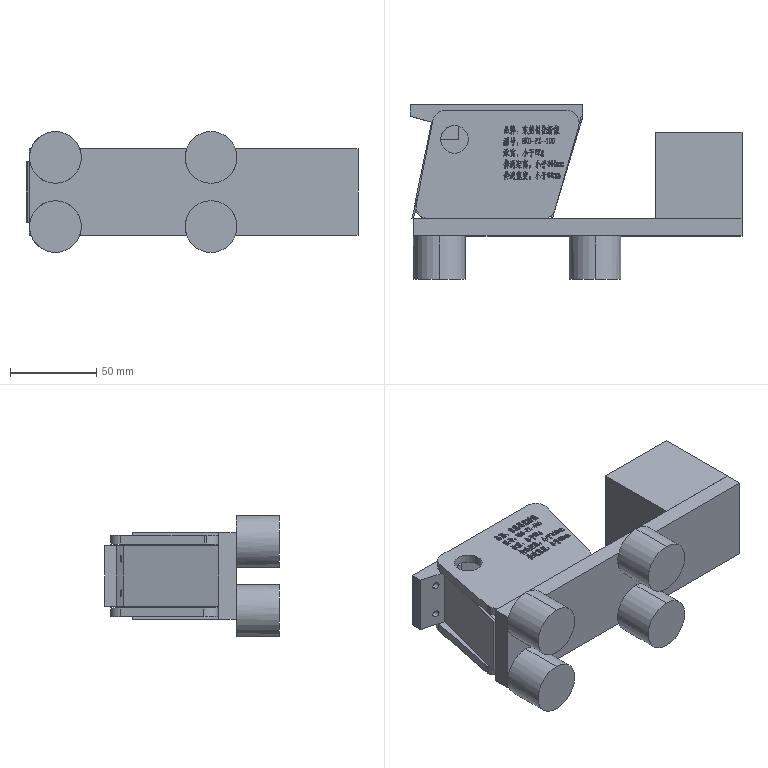Part | STEP file | SKC-PZ-100 counterweight vibratory feeder | 7 solids | 3015 faces | volume 385547 mm3 | plane 2025 | spline 961 | cylinder 29 | commonest cylinder face diameters 14 x10 4 x8 30 x8 16 x3